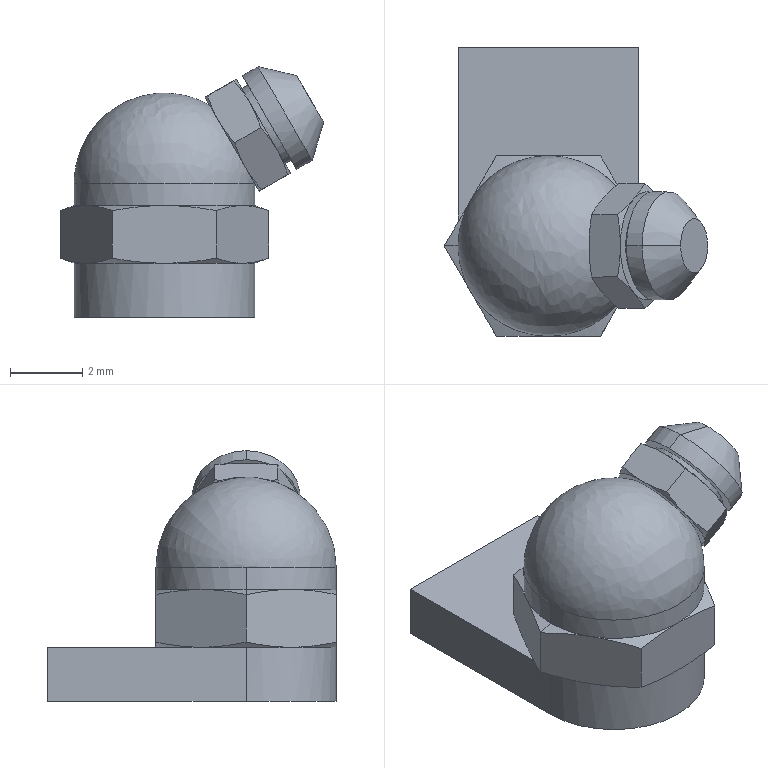Part | STEP file | 13 | 1 solid | 57 faces | box 7.302 x 8 x 6.95 mm | volume 149.976 mm3 | cone 28 | plane 21 | cylinder 7 | spline 1 | commonest cylinder face diameters 5 x3 2.4 x2 3 x2